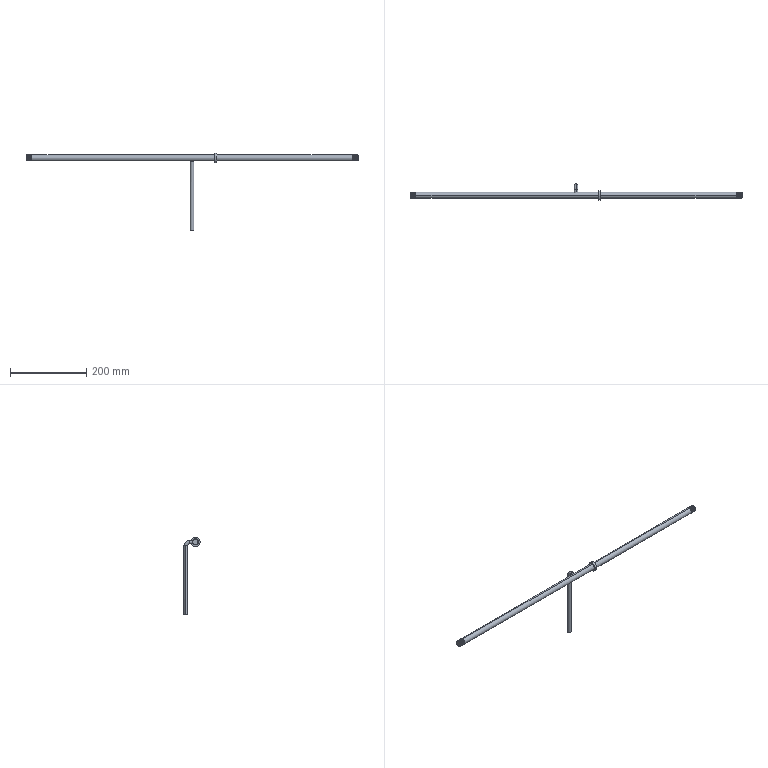Part | SolidWorks | features ICE 2, LPattern 1, MirrorPattern 1, RevCut 1, Sweep 1 | 2 solids | 142 faces | box 870 x 42.5 x 203.5 mm | volume 192112 mm3 | cone 124 | cylinder 10 | plane 6 | torus 2 | commonest cylinder face diameters 10 x4 16 x4 25 x2